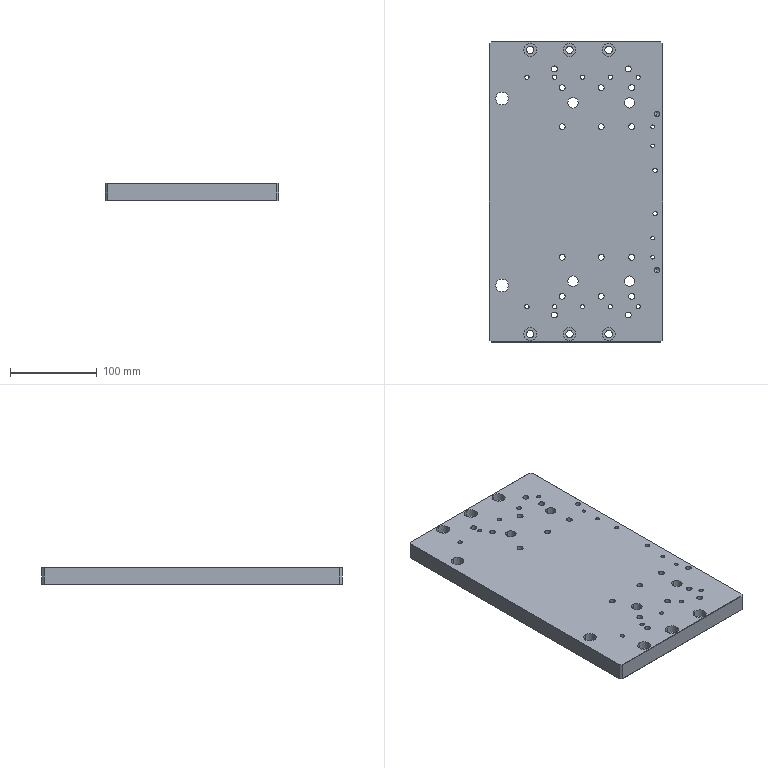NC program | NX | posted with a generic post | part box 200 x 346 x 20 mm
Whole program:
N10 G17 G21 G94 G90
(DRILLING_COPY_1 , TOOL : ZXZ)
N12 T21 M6
N14 G54
N16 G17 G0 G90 X-75. Y95. S3500 M3
N18 G43 Z30. H21
N20 G94 G81 G98 Z-1. F300. R3.
N22 X-53.
N24 X53.
N26 X75.
N28 G80
N30 G0 X75. Y95. Z30.
N32 M5
(DRILLING_COPY_COPY_COPY_COPY_COPY_COPY , TOOL : 3.5ZT)
N34 T07 M6
N36 G54
N38 G17 G0 G90 X-75. Y95. S2000 M3
N40 G43 Z30. H7
N42 G94 G83 G98 Z-9.052 F130. Q2. R3.
N44 X-53.
N46 X53.
N48 X75.
N50 G80
N52 G0 X75. Y95. Z30.
N54 M5
(刀补11_COPY , TOOL : D3)
N56 T03 M6
N58 G54
N60 G17 G0 G90 X-75. Y95. S6578 M3
N62 G43 Z30. H3
N64 Z0.5
N66 G41 G94 G1 X-74.904 Y95.028 F1200. D3
N68 G3 X-75. Y95.44 R0.217
N70 X-75. Y95.44 Z0.4 I0. J-0.44
N72 X-75. Y95.44 Z0.3 I0. J-0.44
N74 X-75. Y95.44 Z0.2 I0. J-0.44
N76 X-75. Y95.44 Z0.1 I0. J-0.44
N78 X-75. Y95.44 Z0. I0. J-0.44
N80 X-75. Y95.44 Z-0.1 I0. J-0.44
N82 X-75. Y95.44 Z-0.2 I0. J-0.44
N84 X-75. Y95.44 Z-0.3 I0. J-0.44
N86 X-75. Y95.44 Z-0.4 I0. J-0.44
N88 X-75. Y95.44 Z-0.5 I0. J-0.44
N90 X-75. Y95.44 Z-0.6 I0. J-0.44
N92 X-75. Y95.44 Z-0.7 I0. J-0.44
N94 X-75. Y95.44 Z-0.8 I0. J-0.44
N96 X-75. Y95.44 Z-0.9 I0. J-0.44
N98 X-75. Y95.44 Z-1. I0. J-0.44
N100 X-75. Y95.44 Z-1.1 I0. J-0.44
N102 X-75. Y95.44 Z-1.2 I0. J-0.44
N104 X-75. Y95.44 Z-1.3 I0. J-0.44
N106 X-75. Y95.44 Z-1.4 I0. J-0.44
N108 X-75. Y95.44 Z-1.5 I0. J-0.44
N110 X-75. Y95.44 Z-1.6 I0. J-0.44
N112 X-75. Y95.44 Z-1.7 I0. J-0.44
N114 X-75. Y95.44 Z-1.8 I0. J-0.44
N116 X-75. Y95.44 Z-1.9 I0. J-0.44
N118 X-75. Y95.44 Z-2. I0. J-0.44
N120 X-75. Y95.44 Z-2.1 I0. J-0.44
N122 X-75. Y95.44 Z-2.2 I0. J-0.44
N124 X-75. Y95.44 Z-2.3 I0. J-0.44
N126 X-75. Y95.44 Z-2.4 I0. J-0.44
N128 X-75. Y95.44 Z-2.5 I0. J-0.44
N130 X-75. Y95.44 Z-2.6 I0. J-0.44
N132 X-75. Y95.44 Z-2.7 I0. J-0.44
N134 X-75. Y95.44 Z-2.8 I0. J-0.44
N136 X-75. Y95.44 Z-2.9 I0. J-0.44
N138 X-75. Y95.44 Z-3. I0. J-0.44
N140 X-75. Y95.44 Z-3.1 I0. J-0.44
N142 X-75. Y95.44 Z-3.2 I0. J-0.44
N144 X-75. Y95.44 Z-3.3 I0. J-0.44
N146 X-75. Y95.44 Z-3.4 I0. J-0.44
N148 X-75. Y95.44 Z-3.5 I0. J-0.44
N150 X-75. Y95.44 Z-3.6 I0. J-0.44
N152 X-75. Y95.44 Z-3.7 I0. J-0.44
N154 X-75. Y95.44 Z-3.8 I0. J-0.44
N156 X-75. Y95.44 Z-3.9 I0. J-0.44
N158 X-75. Y95.44 Z-4. I0. J-0.44
N160 X-75. Y95.44 Z-4.1 I0. J-0.44
N162 X-75. Y95.44 Z-4.2 I0. J-0.44
N164 X-75. Y95.44 Z-4.3 I0. J-0.44
N166 X-75. Y95.44 Z-4.4 I0. J-0.44
N168 X-75. Y95.44 Z-4.5 I0. J-0.44
N170 X-75. Y95.44 Z-4.6 I0. J-0.44
N172 X-75. Y95.44 Z-4.7 I0. J-0.44
N174 X-75. Y95.44 Z-4.8 I0. J-0.44
N176 X-75. Y95.44 Z-4.9 I0. J-0.44
N178 X-75. Y95.44 Z-5. I0. J-0.44
N180 X-75. Y95.44 Z-5.1 I0. J-0.44
N182 X-75. Y95.44 Z-5.2 I0. J-0.44
N184 X-75. Y95.44 Z-5.3 I0. J-0.44
N186 X-75. Y95.44 Z-5.4 I0. J-0.44
N188 X-75. Y95.44 Z-5.5 I0. J-0.44
N190 X-75. Y95.44 Z-5.6 I0. J-0.44
N192 X-75. Y95.44 Z-5.7 I0. J-0.44
N194 X-75. Y95.44 Z-5.8 I0. J-0.44
N196 X-75. Y95.44 Z-5.9 I0. J-0.44
N198 X-75. Y95.44 Z-6. I0. J-0.44
N200 X-75. Y95.44 Z-6.1 I0. J-0.44
N202 X-75. Y95.44 Z-6.2 I0. J-0.44
N204 X-75. Y95.44 Z-6.3 I0. J-0.44
N206 X-75. Y95.44 Z-6.4 I0. J-0.44
N208 X-75. Y95.44 Z-6.5 I0. J-0.44
N210 X-75. Y95.44 Z-6.6 I0. J-0.44
N212 X-75. Y95.44 Z-6.7 I0. J-0.44
N214 X-75. Y95.44 Z-6.8 I0. J-0.44
N216 X-75. Y95.44 Z-6.9 I0. J-0.44
N218 X-75. Y95.44 Z-7. I0. J-0.44
N220 X-75. Y95.44 Z-7.1 I0. J-0.44
N222 X-75. Y95.44 Z-7.2 I0. J-0.44
N224 X-75. Y95.44 Z-7.3 I0. J-0.44
N226 X-75. Y95.44 Z-7.4 I0. J-0.44
N228 X-75. Y95.44 Z-7.5 I0. J-0.44
N230 X-75. Y95.44 Z-7.6 I0. J-0.44
N232 X-75. Y95.44 Z-7.7 I0. J-0.44
N234 X-75. Y95.44 Z-7.8 I0. J-0.44
N236 X-75. Y95.44 Z-7.9 I0. J-0.44
N238 X-75. Y95.44 Z-8. I0. J-0.44
N240 X-75.44 Y95. R0.44
N242 X-75. Y95.44 R-0.44
N244 X-75.096 Y95.028 R0.217
N246 G40
N248 G1 X-75. Y95.
N250 G0 Z30.
N252 X-53.
N254 Z0.5
N256 G41 G1 X-52.904 Y95.028
N258 G3 X-53. Y95.44 R0.217
N260 X-53. Y95.44 Z0.4 I0. J-0.44
N262 X-53. Y95.44 Z0.3 I0. J-0.44
N264 X-53. Y95.44 Z0.2 I0. J-0.44
N266 X-53. Y95.44 Z0.1 I0. J-0.44
N268 X-53. Y95.44 Z0. I0. J-0.44
N270 X-53. Y95.44 Z-0.1 I0. J-0.44
N272 X-53. Y95.44 Z-0.2 I0. J-0.44
N274 X-53. Y95.44 Z-0.3 I0. J-0.44
N276 X-53. Y95.44 Z-0.4 I0. J-0.44
N278 X-53. Y95.44 Z-0.5 I0. J-0.44
N280 X-53. Y95.44 Z-0.6 I0. J-0.44
N282 X-53. Y95.44 Z-0.7 I0. J-0.44
N284 X-53. Y95.44 Z-0.8 I0. J-0.44
N286 X-53. Y95.44 Z-0.9 I0. J-0.44
N288 X-53. Y95.44 Z-1. I0. J-0.44
N290 X-53. Y95.44 Z-1.1 I0. J-0.44
N292 X-53. Y95.44 Z-1.2 I0. J-0.44
N294 X-53. Y95.44 Z-1.3 I0. J-0.44
N296 X-53. Y95.44 Z-1.4 I0. J-0.44
N298 X-53. Y95.44 Z-1.5 I0. J-0.44
N300 X-53. Y95.44 Z-1.6 I0. J-0.44
N302 X-53. Y95.44 Z-1.7 I0. J-0.44
N304 X-53. Y95.44 Z-1.8 I0. J-0.44
N306 X-53. Y95.44 Z-1.9 I0. J-0.44
N308 X-53. Y95.44 Z-2. I0. J-0.44
N310 X-53. Y95.44 Z-2.1 I0. J-0.44
N312 X-53. Y95.44 Z-2.2 I0. J-0.44
N314 X-53. Y95.44 Z-2.3 I0. J-0.44
N316 X-53. Y95.44 Z-2.4 I0. J-0.44
N318 X-53. Y95.44 Z-2.5 I0. J-0.44
N320 X-53. Y95.44 Z-2.6 I0. J-0.44
N322 X-53. Y95.44 Z-2.7 I0. J-0.44
N324 X-53. Y95.44 Z-2.8 I0. J-0.44
N326 X-53. Y95.44 Z-2.9 I0. J-0.44
N328 X-53. Y95.44 Z-3. I0. J-0.44
N330 X-53. Y95.44 Z-3.1 I0. J-0.44
N332 X-53. Y95.44 Z-3.2 I0. J-0.44
N334 X-53. Y95.44 Z-3.3 I0. J-0.44
N336 X-53. Y95.44 Z-3.4 I0. J-0.44
N338 X-53. Y95.44 Z-3.5 I0. J-0.44
N340 X-53. Y95.44 Z-3.6 I0. J-0.44
N342 X-53. Y95.44 Z-3.7 I0. J-0.44
N344 X-53. Y95.44 Z-3.8 I0. J-0.44
N346 X-53. Y95.44 Z-3.9 I0. J-0.44
N348 X-53. Y95.44 Z-4. I0. J-0.44
N350 X-53. Y95.44 Z-4.1 I0. J-0.44
N352 X-53. Y95.44 Z-4.2 I0. J-0.44
N354 X-53. Y95.44 Z-4.3 I0. J-0.44
N356 X-53. Y95.44 Z-4.4 I0. J-0.44
N358 X-53. Y95.44 Z-4.5 I0. J-0.44
N360 X-53. Y95.44 Z-4.6 I0. J-0.44
N362 X-53. Y95.44 Z-4.7 I0. J-0.44
N364 X-53. Y95.44 Z-4.8 I0. J-0.44
N366 X-53. Y95.44 Z-4.9 I0. J-0.44
N368 X-53. Y95.44 Z-5. I0. J-0.44
N370 X-53. Y95.44 Z-5.1 I0. J-0.44
N372 X-53. Y95.44 Z-5.2 I0. J-0.44
N374 X-53. Y95.44 Z-5.3 I0. J-0.44
N376 X-53. Y95.44 Z-5.4 I0. J-0.44
N378 X-53. Y95.44 Z-5.5 I0. J-0.44
N380 X-53. Y95.44 Z-5.6 I0. J-0.44
N382 X-53. Y95.44 Z-5.7 I0. J-0.44
N384 X-53. Y95.44 Z-5.8 I0. J-0.44
N386 X-53. Y95.44 Z-5.9 I0. J-0.44
N388 X-53. Y95.44 Z-6. I0. J-0.44
N390 X-53. Y95.44 Z-6.1 I0. J-0.44
N392 X-53. Y95.44 Z-6.2 I0. J-0.44
N394 X-53. Y95.44 Z-6.3 I0. J-0.44
N396 X-53. Y95.44 Z-6.4 I0. J-0.44
N398 X-53. Y95.44 Z-6.5 I0. J-0.44
N400 X-53. Y95.44 Z-6.6 I0. J-0.44
N402 X-53. Y95.44 Z-6.7 I0. J-0.44
N404 X-53. Y95.44 Z-6.8 I0. J-0.44
N406 X-53. Y95.44 Z-6.9 I0. J-0.44
N408 X-53. Y95.44 Z-7. I0. J-0.44
N410 X-53. Y95.44 Z-7.1 I0. J-0.44
N412 X-53. Y95.44 Z-7.2 I0. J-0.44
N414 X-53. Y95.44 Z-7.3 I0. J-0.44
N416 X-53. Y95.44 Z-7.4 I0. J-0.44
N418 X-53. Y95.44 Z-7.5 I0. J-0.44
N420 X-53. Y95.44 Z-7.6 I0. J-0.44
N422 X-53. Y95.44 Z-7.7 I0. J-0.44
N424 X-53. Y95.44 Z-7.8 I0. J-0.44
N426 X-53. Y95.44 Z-7.9 I0. J-0.44
N428 X-53. Y95.44 Z-8. I0. J-0.44
N430 X-53.44 Y95. R0.44
N432 X-53. Y95.44 R-0.44
N434 X-53.096 Y95.028 R0.217
N436 G40
N438 G1 X-53. Y95.
N440 G0 Z30.
N442 X53.
N444 Z0.5
N446 G41 G1 X53.096 Y95.028
N448 G3 X53. Y95.44 R0.217
N450 X53. Y95.44 Z0.4 I0. J-0.44
N452 X53. Y95.44 Z0.3 I0. J-0.44
N454 X53. Y95.44 Z0.2 I0. J-0.44
N456 X53. Y95.44 Z0.1 I0. J-0.44
N458 X53. Y95.44 Z0. I0. J-0.44
N460 X53. Y95.44 Z-0.1 I0. J-0.44
N462 X53. Y95.44 Z-0.2 I0. J-0.44
N464 X53. Y95.44 Z-0.3 I0. J-0.44
N466 X53. Y95.44 Z-0.4 I0. J-0.44
N468 X53. Y95.44 Z-0.5 I0. J-0.44
N470 X53. Y95.44 Z-0.6 I0. J-0.44
N472 X53. Y95.44 Z-0.7 I0. J-0.44
N474 X53. Y95.44 Z-0.8 I0. J-0.44
N476 X53. Y95.44 Z-0.9 I0. J-0.44
N478 X53. Y95.44 Z-1. I0. J-0.44
N480 X53. Y95.44 Z-1.1 I0. J-0.44
N482 X53. Y95.44 Z-1.2 I0. J-0.44
N484 X53. Y95.44 Z-1.3 I0. J-0.44
N486 X53. Y95.44 Z-1.4 I0. J-0.44
N488 X53. Y95.44 Z-1.5 I0. J-0.44
N490 X53. Y95.44 Z-1.6 I0. J-0.44
N492 X53. Y95.44 Z-1.7 I0. J-0.44
N494 X53. Y95.44 Z-1.8 I0. J-0.44
N496 X53. Y95.44 Z-1.9 I0. J-0.44
N498 X53. Y95.44 Z-2. I0. J-0.44
N500 X53. Y95.44 Z-2.1 I0. J-0.44
N502 X53. Y95.44 Z-2.2 I0. J-0.44
N504 X53. Y95.44 Z-2.3 I0. J-0.44
N506 X53. Y95.44 Z-2.4 I0. J-0.44
N508 X53. Y95.44 Z-2.5 I0. J-0.44
N510 X53. Y95.44 Z-2.6 I0. J-0.44
N512 X53. Y95.44 Z-2.7 I0. J-0.44
N514 X53. Y95.44 Z-2.8 I0. J-0.44
N516 X53. Y95.44 Z-2.9 I0. J-0.44
N518 X53. Y95.44 Z-3. I0. J-0.44
N520 X53. Y95.44 Z-3.1 I0. J-0.44
N522 X53. Y95.44 Z-3.2 I0. J-0.44
N524 X53. Y95.44 Z-3.3 I0. J-0.44
N526 X53. Y95.44 Z-3.4 I0. J-0.44
N528 X53. Y95.44 Z-3.5 I0. J-0.44
N530 X53. Y95.44 Z-3.6 I0. J-0.44
N532 X53. Y95.44 Z-3.7 I0. J-0.44
N534 X53. Y95.44 Z-3.8 I0. J-0.44
N536 X53. Y95.44 Z-3.9 I0. J-0.44
N538 X53. Y95.44 Z-4. I0. J-0.44
N540 X53. Y95.44 Z-4.1 I0. J-0.44
N542 X53. Y95.44 Z-4.2 I0. J-0.44
N544 X53. Y95.44 Z-4.3 I0. J-0.44
N546 X53. Y95.44 Z-4.4 I0. J-0.44
N548 X53. Y95.44 Z-4.5 I0. J-0.44
N550 X53. Y95.44 Z-4.6 I0. J-0.44
N552 X53. Y95.44 Z-4.7 I0. J-0.44
N554 X53. Y95.44 Z-4.8 I0. J-0.44
N556 X53. Y95.44 Z-4.9 I0. J-0.44
N558 X53. Y95.44 Z-5. I0. J-0.44
N560 X53. Y95.44 Z-5.1 I0. J-0.44
N562 X53. Y95.44 Z-5.2 I0. J-0.44
N564 X53. Y95.44 Z-5.3 I0. J-0.44
N566 X53. Y95.44 Z-5.4 I0. J-0.44
N568 X53. Y95.44 Z-5.5 I0. J-0.44
N570 X53. Y95.44 Z-5.6 I0. J-0.44
N572 X53. Y95.44 Z-5.7 I0. J-0.44
N574 X53. Y95.44 Z-5.8 I0. J-0.44
N576 X53. Y95.44 Z-5.9 I0. J-0.44
N578 X53. Y95.44 Z-6. I0. J-0.44
N580 X53. Y95.44 Z-6.1 I0. J-0.44
N582 X53. Y95.44 Z-6.2 I0. J-0.44
N584 X53. Y95.44 Z-6.3 I0. J-0.44
N586 X53. Y95.44 Z-6.4 I0. J-0.44
N588 X53. Y95.44 Z-6.5 I0. J-0.44
N590 X53. Y95.44 Z-6.6 I0. J-0.44
N592 X53. Y95.44 Z-6.7 I0. J-0.44
N594 X53. Y95.44 Z-6.8 I0. J-0.44
N596 X53. Y95.44 Z-6.9 I0. J-0.44
N598 X53. Y95.44 Z-7. I0. J-0.44
N600 X53. Y95.44 Z-7.1 I0. J-0.44
N602 X53. Y95.44 Z-7.2 I0. J-0.44
N604 X53. Y95.44 Z-7.3 I0. J-0.44
N606 X53. Y95.44 Z-7.4 I0. J-0.44
N608 X53. Y95.44 Z-7.5 I0. J-0.44
N610 X53. Y95.44 Z-7.6 I0. J-0.44
N612 X53. Y95.44 Z-7.7 I0. J-0.44
N614 X53. Y95.44 Z-7.8 I0. J-0.44
N616 X53. Y95.44 Z-7.9 I0. J-0.44
N618 X53. Y95.44 Z-8. I0. J-0.44
N620 X52.56 Y95. R0.44
N622 X53. Y95.44 R-0.44
N624 X52.904 Y95.028 R0.217
N626 G40
N628 G1 X53. Y95.
N630 G0 Z30.
N632 X75.
N634 Z0.5
N636 G41 G1 X75.096 Y95.028
N638 G3 X75. Y95.44 R0.217
N640 X75. Y95.44 Z0.4 I0. J-0.44
N642 X75. Y95.44 Z0.3 I0. J-0.44
N644 X75. Y95.44 Z0.2 I0. J-0.44
N646 X75. Y95.44 Z0.1 I0. J-0.44
N648 X75. Y95.44 Z0. I0. J-0.44
N650 X75. Y95.44 Z-0.1 I0. J-0.44
N652 X75. Y95.44 Z-0.2 I0. J-0.44
N654 X75. Y95.44 Z-0.3 I0. J-0.44
N656 X75. Y95.44 Z-0.4 I0. J-0.44
N658 X75. Y95.44 Z-0.5 I0. J-0.44
N660 X75. Y95.44 Z-0.6 I0. J-0.44
N662 X75. Y95.44 Z-0.7 I0. J-0.44
N664 X75. Y95.44 Z-0.8 I0. J-0.44
N666 X75. Y95.44 Z-0.9 I0. J-0.44
N668 X75. Y95.44 Z-1. I0. J-0.44
N670 X75. Y95.44 Z-1.1 I0. J-0.44
N672 X75. Y95.44 Z-1.2 I0. J-0.44
N674 X75. Y95.44 Z-1.3 I0. J-0.44
N676 X75. Y95.44 Z-1.4 I0. J-0.44
N678 X75. Y95.44 Z-1.5 I0. J-0.44
N680 X75. Y95.44 Z-1.6 I0. J-0.44
N682 X75. Y95.44 Z-1.7 I0. J-0.44
N684 X75. Y95.44 Z-1.8 I0. J-0.44
N686 X75. Y95.44 Z-1.9 I0. J-0.44
N688 X75. Y95.44 Z-2. I0. J-0.44
N690 X75. Y95.44 Z-2.1 I0. J-0.44
N692 X75. Y95.44 Z-2.2 I0. J-0.44
N694 X75. Y95.44 Z-2.3 I0. J-0.44
N696 X75. Y95.44 Z-2.4 I0. J-0.44
N698 X75. Y95.44 Z-2.5 I0. J-0.44
N700 X75. Y95.44 Z-2.6 I0. J-0.44
N702 X75. Y95.44 Z-2.7 I0. J-0.44
N704 X75. Y95.44 Z-2.8 I0. J-0.44
N706 X75. Y95.44 Z-2.9 I0. J-0.44
N708 X75. Y95.44 Z-3. I0. J-0.44
N710 X75. Y95.44 Z-3.1 I0. J-0.44
N712 X75. Y95.44 Z-3.2 I0. J-0.44
N714 X75. Y95.44 Z-3.3 I0. J-0.44
N716 X75. Y95.44 Z-3.4 I0. J-0.44
N718 X75. Y95.44 Z-3.5 I0. J-0.44
N720 X75. Y95.44 Z-3.6 I0. J-0.44
N722 X75. Y95.44 Z-3.7 I0. J-0.44
N724 X75. Y95.44 Z-3.8 I0. J-0.44
N726 X75. Y95.44 Z-3.9 I0. J-0.44
N728 X75. Y95.44 Z-4. I0. J-0.44
N730 X75. Y95.44 Z-4.1 I0. J-0.44
N732 X75. Y95.44 Z-4.2 I0. J-0.44
N734 X75. Y95.44 Z-4.3 I0. J-0.44
N736 X75. Y95.44 Z-4.4 I0. J-0.44
N738 X75. Y95.44 Z-4.5 I0. J-0.44
N740 X75. Y95.44 Z-4.6 I0. J-0.44
N742 X75. Y95.44 Z-4.7 I0. J-0.44
N744 X75. Y95.44 Z-4.8 I0. J-0.44
N746 X75. Y95.44 Z-4.9 I0. J-0.44
N748 X75. Y95.44 Z-5. I0. J-0.44
N750 X75. Y95.44 Z-5.1 I0. J-0.44
N752 X75. Y95.44 Z-5.2 I0. J-0.44
N754 X75. Y95.44 Z-5.3 I0. J-0.44
N756 X75. Y95.44 Z-5.4 I0. J-0.44
N758 X75. Y95.44 Z-5.5 I0. J-0.44
N760 X75. Y95.44 Z-5.6 I0. J-0.44
N762 X75. Y95.44 Z-5.7 I0. J-0.44
N764 X75. Y95.44 Z-5.8 I0. J-0.44
N766 X75. Y95.44 Z-5.9 I0. J-0.44
N768 X75. Y95.44 Z-6. I0. J-0.44
N770 X75. Y95.44 Z-6.1 I0. J-0.44
N772 X75. Y95.44 Z-6.2 I0. J-0.44
N774 X75. Y95.44 Z-6.3 I0. J-0.44
N776 X75. Y95.44 Z-6.4 I0. J-0.44
N778 X75. Y95.44 Z-6.5 I0. J-0.44
N780 X75. Y95.44 Z-6.6 I0. J-0.44
N782 X75. Y95.44 Z-6.7 I0. J-0.44
N784 X75. Y95.44 Z-6.8 I0. J-0.44
N786 X75. Y95.44 Z-6.9 I0. J-0.44
N788 X75. Y95.44 Z-7. I0. J-0.44
N790 X75. Y95.44 Z-7.1 I0. J-0.44
N792 X75. Y95.44 Z-7.2 I0. J-0.44
N794 X75. Y95.44 Z-7.3 I0. J-0.44
N796 X75. Y95.44 Z-7.4 I0. J-0.44
N798 X75. Y95.44 Z-7.5 I0. J-0.44
N800 X75. Y95.44 Z-7.6 I0. J-0.44
N802 X75. Y95.44 Z-7.7 I0. J-0.44
N804 X75. Y95.44 Z-7.8 I0. J-0.44
N806 X75. Y95.44 Z-7.9 I0. J-0.44
N808 X75. Y95.44 Z-8. I0. J-0.44
N810 X74.56 Y95. R0.44
N812 X75. Y95.44 R-0.44
N814 X74.904 Y95.028 R0.217
N816 G40
N818 G1 X75. Y95.
N820 G0 Z30.
N822 M5
N824 M2